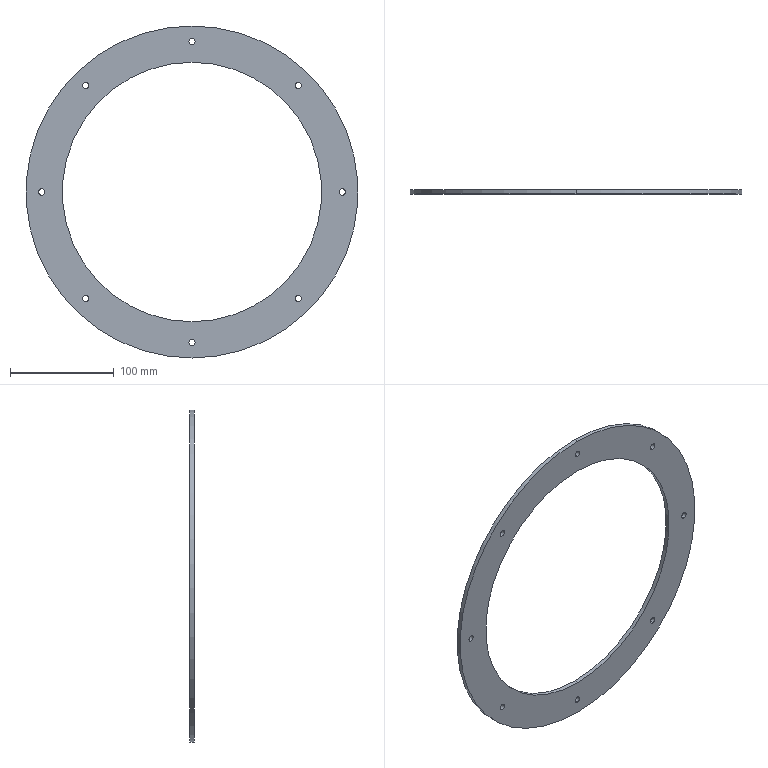Part | SolidWorks | features CirPattern 1, Extrusion 1, ICE 1 | 1 solid | 22 faces | box 320 x 4 x 320 mm | volume 124445 mm3 | cylinder 20 | plane 2 | commonest cylinder face diameters 6 x16 250 x2 320 x2
STEP:
#1=CARTESIAN_POINT('',(-102.53,0.,-105.53));
#2=VERTEX_POINT('',#1);
#3=CARTESIAN_POINT('',(-102.53,0.,-99.53));
#4=VERTEX_POINT('',#3);
#5=CARTESIAN_POINT('',(-102.53,0.,-102.53));
#6=DIRECTION('',(0.,1.,0.));
#7=DIRECTION('',(0.7071,0.,0.7071));
#8=AXIS2_PLACEMENT_3D('',#5,#6,#7);
#9=CIRCLE('',#8,3.);
#10=EDGE_CURVE('',#2,#4,#9,.T.);
#11=ORIENTED_EDGE('',*,*,#10,.F.);
#12=CARTESIAN_POINT('',(-102.53,4.,-105.53));
#13=VERTEX_POINT('',#12);
#14=CARTESIAN_POINT('',(-102.53,0.,-105.53));
#15=DIRECTION('',(0.,1.,0.));
#16=VECTOR('',#15,1000.);
#17=LINE('',#14,#16);
#18=EDGE_CURVE('',#2,#13,#17,.T.);
#19=ORIENTED_EDGE('',*,*,#18,.T.);
#20=CARTESIAN_POINT('',(-102.53,4.,-99.53));
#21=VERTEX_POINT('',#20);
#22=CARTESIAN_POINT('',(-102.53,4.,-102.53));
#23=DIRECTION('',(0.,1.,0.));
#24=DIRECTION('',(0.7071,0.,0.7071));
#25=AXIS2_PLACEMENT_3D('',#22,#23,#24);
#26=CIRCLE('',#25,3.);
#27=EDGE_CURVE('',#13,#21,#26,.T.);
#28=ORIENTED_EDGE('',*,*,#27,.T.);
#29=CARTESIAN_POINT('',(-102.53,0.,-99.53));
#30=DIRECTION('',(0.,1.,0.));
#31=VECTOR('',#30,1000.);
#32=LINE('',#29,#31);
#33=EDGE_CURVE('',#4,#21,#32,.T.);
#34=ORIENTED_EDGE('',*,*,#33,.F.);
#35=EDGE_LOOP('',(#11,#19,#28,#34));
#36=FACE_OUTER_BOUND('',#35,.T.);
#37=CARTESIAN_POINT('',(-102.53,0.,-102.53));
#38=DIRECTION('',(0.,1.,0.));
#39=DIRECTION('',(0.,0.,1.));
#40=AXIS2_PLACEMENT_3D('',#37,#38,#39);
#41=CYLINDRICAL_SURFACE('',#40,3.);
#42=ADVANCED_FACE('',(#36),#41,.F.);
#43=CARTESIAN_POINT('',(-145.,0.,-3.));
#44=VERTEX_POINT('',#43);
#45=CARTESIAN_POINT('',(-145.,0.,3.));
#46=VERTEX_POINT('',#45);
#47=CARTESIAN_POINT('',(-145.,0.,0.));
#48=DIRECTION('',(0.,1.,0.));
#49=DIRECTION('',(1.,0.,0.));
#50=AXIS2_PLACEMENT_3D('',#47,#48,#49);
#51=CIRCLE('',#50,3.);
#52=EDGE_CURVE('',#44,#46,#51,.T.);
#53=ORIENTED_EDGE('',*,*,#52,.F.);
#54=CARTESIAN_POINT('',(-145.,4.,-3.));
#55=VERTEX_POINT('',#54);
#56=CARTESIAN_POINT('',(-145.,0.,-3.));
#57=DIRECTION('',(0.,1.,0.));
#58=VECTOR('',#57,1000.);
#59=LINE('',#56,#58);
#60=EDGE_CURVE('',#44,#55,#59,.T.);
#61=ORIENTED_EDGE('',*,*,#60,.T.);
#62=CARTESIAN_POINT('',(-145.,4.,3.));
#63=VERTEX_POINT('',#62);
#64=CARTESIAN_POINT('',(-145.,4.,0.));
#65=DIRECTION('',(0.,1.,0.));
#66=DIRECTION('',(1.,0.,0.));
#67=AXIS2_PLACEMENT_3D('',#64,#65,#66);
#68=CIRCLE('',#67,3.);
#69=EDGE_CURVE('',#55,#63,#68,.T.);
#70=ORIENTED_EDGE('',*,*,#69,.T.);
#71=CARTESIAN_POINT('',(-145.,0.,3.));
#72=DIRECTION('',(0.,1.,0.));
#73=VECTOR('',#72,1000.);
#74=LINE('',#71,#73);
#75=EDGE_CURVE('',#46,#63,#74,.T.);
#76=ORIENTED_EDGE('',*,*,#75,.F.);
#77=EDGE_LOOP('',(#53,#61,#70,#76));
#78=FACE_OUTER_BOUND('',#77,.T.);
#79=CARTESIAN_POINT('',(-145.,0.,0.));
#80=DIRECTION('',(0.,1.,0.));
#81=DIRECTION('',(0.,0.,1.));
#82=AXIS2_PLACEMENT_3D('',#79,#80,#81);
#83=CYLINDRICAL_SURFACE('',#82,3.);
#84=ADVANCED_FACE('',(#78),#83,.F.);
#85=CARTESIAN_POINT('',(-102.53,0.,99.53));
#86=VERTEX_POINT('',#85);
#87=CARTESIAN_POINT('',(-102.53,0.,105.53));
#88=VERTEX_POINT('',#87);
#89=CARTESIAN_POINT('',(-102.53,0.,102.53));
#90=DIRECTION('',(0.,1.,0.));
#91=DIRECTION('',(0.7071,0.,-0.7071));
#92=AXIS2_PLACEMENT_3D('',#89,#90,#91);
#93=CIRCLE('',#92,3.);
#94=EDGE_CURVE('',#86,#88,#93,.T.);
#95=ORIENTED_EDGE('',*,*,#94,.F.);
#96=CARTESIAN_POINT('',(-102.53,4.,99.53));
#97=VERTEX_POINT('',#96);
#98=CARTESIAN_POINT('',(-102.53,0.,99.53));
#99=DIRECTION('',(0.,1.,0.));
#100=VECTOR('',#99,1000.);
#101=LINE('',#98,#100);
#102=EDGE_CURVE('',#86,#97,#101,.T.);
#103=ORIENTED_EDGE('',*,*,#102,.T.);
#104=CARTESIAN_POINT('',(-102.53,4.,105.53));
#105=VERTEX_POINT('',#104);
#106=CARTESIAN_POINT('',(-102.53,4.,102.53));
#107=DIRECTION('',(0.,1.,0.));
#108=DIRECTION('',(0.7071,0.,-0.7071));
#109=AXIS2_PLACEMENT_3D('',#106,#107,#108);
#110=CIRCLE('',#109,3.);
#111=EDGE_CURVE('',#97,#105,#110,.T.);
#112=ORIENTED_EDGE('',*,*,#111,.T.);
#113=CARTESIAN_POINT('',(-102.53,0.,105.53));
#114=DIRECTION('',(0.,1.,0.));
#115=VECTOR('',#114,1000.);
#116=LINE('',#113,#115);
#117=EDGE_CURVE('',#88,#105,#116,.T.);
#118=ORIENTED_EDGE('',*,*,#117,.F.);
#119=EDGE_LOOP('',(#95,#103,#112,#118));
#120=FACE_OUTER_BOUND('',#119,.T.);
#121=CARTESIAN_POINT('',(-102.53,0.,102.53));
#122=DIRECTION('',(0.,1.,0.));
#123=DIRECTION('',(0.,0.,1.));
#124=AXIS2_PLACEMENT_3D('',#121,#122,#123);
#125=CYLINDRICAL_SURFACE('',#124,3.);
#126=ADVANCED_FACE('',(#120),#125,.F.);
#127=CARTESIAN_POINT('',(0.,0.,142.));
#128=VERTEX_POINT('',#127);
#129=CARTESIAN_POINT('',(0.,0.,148.));
#130=VERTEX_POINT('',#129);
#131=CARTESIAN_POINT('',(0.,0.,145.));
#132=DIRECTION('',(0.,1.,0.));
#133=DIRECTION('',(0.,0.,-1.));
#134=AXIS2_PLACEMENT_3D('',#131,#132,#133);
#135=CIRCLE('',#134,3.);
#136=EDGE_CURVE('',#128,#130,#135,.T.);
#137=ORIENTED_EDGE('',*,*,#136,.F.);
#138=CARTESIAN_POINT('',(0.,4.,142.));
#139=VERTEX_POINT('',#138);
#140=CARTESIAN_POINT('',(0.,0.,142.));
#141=DIRECTION('',(0.,1.,0.));
#142=VECTOR('',#141,1000.);
#143=LINE('',#140,#142);
#144=EDGE_CURVE('',#128,#139,#143,.T.);
#145=ORIENTED_EDGE('',*,*,#144,.T.);
#146=CARTESIAN_POINT('',(0.,4.,148.));
#147=VERTEX_POINT('',#146);
#148=CARTESIAN_POINT('',(0.,4.,145.));
#149=DIRECTION('',(0.,1.,0.));
#150=DIRECTION('',(0.,0.,-1.));
#151=AXIS2_PLACEMENT_3D('',#148,#149,#150);
#152=CIRCLE('',#151,3.);
#153=EDGE_CURVE('',#139,#147,#152,.T.);
#154=ORIENTED_EDGE('',*,*,#153,.T.);
#155=CARTESIAN_POINT('',(0.,0.,148.));
#156=DIRECTION('',(0.,1.,0.));
#157=VECTOR('',#156,1000.);
#158=LINE('',#155,#157);
#159=EDGE_CURVE('',#130,#147,#158,.T.);
#160=ORIENTED_EDGE('',*,*,#159,.F.);
#161=EDGE_LOOP('',(#137,#145,#154,#160));
#162=FACE_OUTER_BOUND('',#161,.T.);
#163=CARTESIAN_POINT('',(0.,0.,145.));
#164=DIRECTION('',(0.,1.,0.));
#165=DIRECTION('',(0.,0.,1.));
#166=AXIS2_PLACEMENT_3D('',#163,#164,#165);
#167=CYLINDRICAL_SURFACE('',#166,3.);
#168=ADVANCED_FACE('',(#162),#167,.F.);
#169=CARTESIAN_POINT('',(102.53,0.,99.53));
#170=VERTEX_POINT('',#169);
#171=CARTESIAN_POINT('',(102.53,0.,105.53));
#172=VERTEX_POINT('',#171);
#173=CARTESIAN_POINT('',(102.53,0.,102.53));
#174=DIRECTION('',(0.,1.,0.));
#175=DIRECTION('',(-0.7071,0.,-0.7071));
#176=AXIS2_PLACEMENT_3D('',#173,#174,#175);
#177=CIRCLE('',#176,3.);
#178=EDGE_CURVE('',#170,#172,#177,.T.);
#179=ORIENTED_EDGE('',*,*,#178,.F.);
#180=CARTESIAN_POINT('',(102.53,4.,99.53));
#181=VERTEX_POINT('',#180);
#182=CARTESIAN_POINT('',(102.53,0.,99.53));
#183=DIRECTION('',(0.,1.,0.));
#184=VECTOR('',#183,1000.);
#185=LINE('',#182,#184);
#186=EDGE_CURVE('',#170,#181,#185,.T.);
#187=ORIENTED_EDGE('',*,*,#186,.T.);
#188=CARTESIAN_POINT('',(102.53,4.,105.53));
#189=VERTEX_POINT('',#188);
#190=CARTESIAN_POINT('',(102.53,4.,102.53));
#191=DIRECTION('',(0.,1.,0.));
#192=DIRECTION('',(-0.7071,0.,-0.7071));
#193=AXIS2_PLACEMENT_3D('',#190,#191,#192);
#194=CIRCLE('',#193,3.);
#195=EDGE_CURVE('',#181,#189,#194,.T.);
#196=ORIENTED_EDGE('',*,*,#195,.T.);
#197=CARTESIAN_POINT('',(102.53,0.,105.53));
#198=DIRECTION('',(0.,1.,0.));
#199=VECTOR('',#198,1000.);
#200=LINE('',#197,#199);
#201=EDGE_CURVE('',#172,#189,#200,.T.);
#202=ORIENTED_EDGE('',*,*,#201,.F.);
#203=EDGE_LOOP('',(#179,#187,#196,#202));
#204=FACE_OUTER_BOUND('',#203,.T.);
#205=CARTESIAN_POINT('',(102.53,0.,102.53));
#206=DIRECTION('',(0.,1.,0.));
#207=DIRECTION('',(0.,0.,1.));
#208=AXIS2_PLACEMENT_3D('',#205,#206,#207);
#209=CYLINDRICAL_SURFACE('',#208,3.);
#210=ADVANCED_FACE('',(#204),#209,.F.);
#211=CARTESIAN_POINT('',(145.,0.,-3.));
#212=VERTEX_POINT('',#211);
#213=CARTESIAN_POINT('',(145.,0.,3.));
#214=VERTEX_POINT('',#213);
#215=CARTESIAN_POINT('',(145.,0.,0.));
#216=DIRECTION('',(0.,1.,0.));
#217=DIRECTION('',(-1.,0.,0.));
#218=AXIS2_PLACEMENT_3D('',#215,#216,#217);
#219=CIRCLE('',#218,3.);
#220=EDGE_CURVE('',#212,#214,#219,.T.);
#221=ORIENTED_EDGE('',*,*,#220,.F.);
#222=CARTESIAN_POINT('',(145.,4.,-3.));
#223=VERTEX_POINT('',#222);
#224=CARTESIAN_POINT('',(145.,0.,-3.));
#225=DIRECTION('',(0.,1.,0.));
#226=VECTOR('',#225,1000.);
#227=LINE('',#224,#226);
#228=EDGE_CURVE('',#212,#223,#227,.T.);
#229=ORIENTED_EDGE('',*,*,#228,.T.);
#230=CARTESIAN_POINT('',(145.,4.,3.));
#231=VERTEX_POINT('',#230);
#232=CARTESIAN_POINT('',(145.,4.,0.));
#233=DIRECTION('',(0.,1.,0.));
#234=DIRECTION('',(-1.,0.,0.));
#235=AXIS2_PLACEMENT_3D('',#232,#233,#234);
#236=CIRCLE('',#235,3.);
#237=EDGE_CURVE('',#223,#231,#236,.T.);
#238=ORIENTED_EDGE('',*,*,#237,.T.);
#239=CARTESIAN_POINT('',(145.,0.,3.));
#240=DIRECTION('',(0.,1.,0.));
#241=VECTOR('',#240,1000.);
#242=LINE('',#239,#241);
#243=EDGE_CURVE('',#214,#231,#242,.T.);
#244=ORIENTED_EDGE('',*,*,#243,.F.);
#245=EDGE_LOOP('',(#221,#229,#238,#244));
#246=FACE_OUTER_BOUND('',#245,.T.);
#247=CARTESIAN_POINT('',(145.,0.,0.));
#248=DIRECTION('',(0.,1.,0.));
#249=DIRECTION('',(0.,0.,1.));
#250=AXIS2_PLACEMENT_3D('',#247,#248,#249);
#251=CYLINDRICAL_SURFACE('',#250,3.);
#252=ADVANCED_FACE('',(#246),#251,.F.);
#253=CARTESIAN_POINT('',(102.53,0.,-105.53));
#254=VERTEX_POINT('',#253);
#255=CARTESIAN_POINT('',(102.53,0.,-99.53));
#256=VERTEX_POINT('',#255);
#257=CARTESIAN_POINT('',(102.53,0.,-102.53));
#258=DIRECTION('',(0.,1.,0.));
#259=DIRECTION('',(-0.7071,0.,0.7071));
#260=AXIS2_PLACEMENT_3D('',#257,#258,#259);
#261=CIRCLE('',#260,3.);
#262=EDGE_CURVE('',#254,#256,#261,.T.);
#263=ORIENTED_EDGE('',*,*,#262,.F.);
#264=CARTESIAN_POINT('',(102.53,4.,-105.53));
#265=VERTEX_POINT('',#264);
#266=CARTESIAN_POINT('',(102.53,0.,-105.53));
#267=DIRECTION('',(0.,1.,0.));
#268=VECTOR('',#267,1000.);
#269=LINE('',#266,#268);
#270=EDGE_CURVE('',#254,#265,#269,.T.);
#271=ORIENTED_EDGE('',*,*,#270,.T.);
#272=CARTESIAN_POINT('',(102.53,4.,-99.53));
#273=VERTEX_POINT('',#272);
#274=CARTESIAN_POINT('',(102.53,4.,-102.53));
#275=DIRECTION('',(0.,1.,0.));
#276=DIRECTION('',(-0.7071,0.,0.7071));
#277=AXIS2_PLACEMENT_3D('',#274,#275,#276);
#278=CIRCLE('',#277,3.);
#279=EDGE_CURVE('',#265,#273,#278,.T.);
#280=ORIENTED_EDGE('',*,*,#279,.T.);
#281=CARTESIAN_POINT('',(102.53,0.,-99.53));
#282=DIRECTION('',(0.,1.,0.));
#283=VECTOR('',#282,1000.);
#284=LINE('',#281,#283);
#285=EDGE_CURVE('',#256,#273,#284,.T.);
#286=ORIENTED_EDGE('',*,*,#285,.F.);
#287=EDGE_LOOP('',(#263,#271,#280,#286));
#288=FACE_OUTER_BOUND('',#287,.T.);
#289=CARTESIAN_POINT('',(102.53,0.,-102.53));
#290=DIRECTION('',(0.,1.,0.));
#291=DIRECTION('',(0.,0.,1.));
#292=AXIS2_PLACEMENT_3D('',#289,#290,#291);
#293=CYLINDRICAL_SURFACE('',#292,3.);
#294=ADVANCED_FACE('',(#288),#293,.F.);
#295=CARTESIAN_POINT('',(0.,0.,-148.));
#296=VERTEX_POINT('',#295);
#297=CARTESIAN_POINT('',(0.,0.,-142.));
#298=VERTEX_POINT('',#297);
#299=CARTESIAN_POINT('',(0.,0.,-145.));
#300=DIRECTION('',(0.,1.,0.));
#301=DIRECTION('',(0.,0.,1.));
#302=AXIS2_PLACEMENT_3D('',#299,#300,#301);
#303=CIRCLE('',#302,3.);
#304=EDGE_CURVE('',#296,#298,#303,.T.);
#305=ORIENTED_EDGE('',*,*,#304,.F.);
#306=CARTESIAN_POINT('',(0.,4.,-148.));
#307=VERTEX_POINT('',#306);
#308=CARTESIAN_POINT('',(0.,0.,-148.));
#309=DIRECTION('',(0.,1.,0.));
#310=VECTOR('',#309,1000.);
#311=LINE('',#308,#310);
#312=EDGE_CURVE('',#296,#307,#311,.T.);
#313=ORIENTED_EDGE('',*,*,#312,.T.);
#314=CARTESIAN_POINT('',(0.,4.,-142.));
#315=VERTEX_POINT('',#314);
#316=CARTESIAN_POINT('',(0.,4.,-145.));
#317=DIRECTION('',(0.,1.,0.));
#318=DIRECTION('',(0.,0.,1.));
#319=AXIS2_PLACEMENT_3D('',#316,#317,#318);
#320=CIRCLE('',#319,3.);
#321=EDGE_CURVE('',#307,#315,#320,.T.);
#322=ORIENTED_EDGE('',*,*,#321,.T.);
#323=CARTESIAN_POINT('',(0.,0.,-142.));
#324=DIRECTION('',(0.,1.,0.));
#325=VECTOR('',#324,1000.);
#326=LINE('',#323,#325);
#327=EDGE_CURVE('',#298,#315,#326,.T.);
#328=ORIENTED_EDGE('',*,*,#327,.F.);
#329=EDGE_LOOP('',(#305,#313,#322,#328));
#330=FACE_OUTER_BOUND('',#329,.T.);
#331=CARTESIAN_POINT('',(0.,0.,-145.));
#332=DIRECTION('',(0.,1.,0.));
#333=DIRECTION('',(0.,0.,1.));
#334=AXIS2_PLACEMENT_3D('',#331,#332,#333);
#335=CYLINDRICAL_SURFACE('',#334,3.);
#336=ADVANCED_FACE('',(#330),#335,.F.);
#337=CARTESIAN_POINT('',(0.,4.,-125.));
#338=VERTEX_POINT('',#337);
#339=CARTESIAN_POINT('',(0.,4.,125.));
#340=VERTEX_POINT('',#339);
#341=CARTESIAN_POINT('',(0.,4.,0.));
#342=DIRECTION('',(0.,1.,0.));
#343=DIRECTION('',(0.,0.,1.));
#344=AXIS2_PLACEMENT_3D('',#341,#342,#343);
#345=CIRCLE('',#344,125.);
#346=EDGE_CURVE('',#338,#340,#345,.T.);
#347=ORIENTED_EDGE('',*,*,#346,.T.);
#348=CARTESIAN_POINT('',(0.,0.,125.));
#349=VERTEX_POINT('',#348);
#350=CARTESIAN_POINT('',(0.,4.,125.));
#351=DIRECTION('',(0.,-1.,0.));
#352=VECTOR('',#351,1000.);
#353=LINE('',#350,#352);
#354=EDGE_CURVE('',#340,#349,#353,.T.);
#355=ORIENTED_EDGE('',*,*,#354,.T.);
#356=CARTESIAN_POINT('',(0.,0.,-125.));
#357=VERTEX_POINT('',#356);
#358=CARTESIAN_POINT('',(0.,0.,0.));
#359=DIRECTION('',(0.,1.,0.));
#360=DIRECTION('',(0.,0.,1.));
#361=AXIS2_PLACEMENT_3D('',#358,#359,#360);
#362=CIRCLE('',#361,125.);
#363=EDGE_CURVE('',#357,#349,#362,.T.);
#364=ORIENTED_EDGE('',*,*,#363,.F.);
#365=CARTESIAN_POINT('',(0.,4.,-125.));
#366=DIRECTION('',(0.,-1.,0.));
#367=VECTOR('',#366,1000.);
#368=LINE('',#365,#367);
#369=EDGE_CURVE('',#338,#357,#368,.T.);
#370=ORIENTED_EDGE('',*,*,#369,.F.);
#371=EDGE_LOOP('',(#347,#355,#364,#370));
#372=FACE_OUTER_BOUND('',#371,.T.);
#373=CARTESIAN_POINT('',(0.,4.,0.));
#374=DIRECTION('',(0.,-1.,0.));
#375=DIRECTION('',(0.,0.,-1.));
#376=AXIS2_PLACEMENT_3D('',#373,#374,#375);
#377=CYLINDRICAL_SURFACE('',#376,125.);
#378=ADVANCED_FACE('',(#372),#377,.F.);
#379=CARTESIAN_POINT('',(0.,4.,160.));
#380=VERTEX_POINT('',#379);
#381=CARTESIAN_POINT('',(0.,4.,-160.));
#382=VERTEX_POINT('',#381);
#383=CARTESIAN_POINT('',(0.,4.,0.));
#384=DIRECTION('',(0.,1.,0.));
#385=DIRECTION('',(0.,0.,1.));
#386=AXIS2_PLACEMENT_3D('',#383,#384,#385);
#387=CIRCLE('',#386,160.);
#388=EDGE_CURVE('',#380,#382,#387,.T.);
#389=ORIENTED_EDGE('',*,*,#388,.F.);
#390=CARTESIAN_POINT('',(0.,0.,160.));
#391=VERTEX_POINT('',#390);
#392=CARTESIAN_POINT('',(0.,4.,160.));
#393=DIRECTION('',(0.,-1.,0.));
#394=VECTOR('',#393,1000.);
#395=LINE('',#392,#394);
#396=EDGE_CURVE('',#380,#391,#395,.T.);
#397=ORIENTED_EDGE('',*,*,#396,.T.);
#398=CARTESIAN_POINT('',(0.,0.,-160.));
#399=VERTEX_POINT('',#398);
#400=CARTESIAN_POINT('',(0.,0.,0.));
#401=DIRECTION('',(0.,1.,0.));
#402=DIRECTION('',(0.,0.,1.));
#403=AXIS2_PLACEMENT_3D('',#400,#401,#402);
#404=CIRCLE('',#403,160.);
#405=EDGE_CURVE('',#391,#399,#404,.T.);
#406=ORIENTED_EDGE('',*,*,#405,.T.);
#407=CARTESIAN_POINT('',(0.,4.,-160.));
#408=DIRECTION('',(0.,-1.,0.));
#409=VECTOR('',#408,1000.);
#410=LINE('',#407,#409);
#411=EDGE_CURVE('',#382,#399,#410,.T.);
#412=ORIENTED_EDGE('',*,*,#411,.F.);
#413=EDGE_LOOP('',(#389,#397,#406,#412));
#414=FACE_OUTER_BOUND('',#413,.T.);
#415=CARTESIAN_POINT('',(0.,4.,0.));
#416=DIRECTION('',(0.,-1.,0.));
#417=DIRECTION('',(0.,0.,-1.));
#418=AXIS2_PLACEMENT_3D('',#415,#416,#417);
#419=CYLINDRICAL_SURFACE('',#418,160.);
#420=ADVANCED_FACE('',(#414),#419,.T.);
#421=CARTESIAN_POINT('',(-102.53,4.,-102.53));
#422=DIRECTION('',(0.,1.,0.));
#423=DIRECTION('',(0.7071,0.,0.7071));
#424=AXIS2_PLACEMENT_3D('',#421,#422,#423);
#425=CIRCLE('',#424,3.);
#426=EDGE_CURVE('',#21,#13,#425,.T.);
#427=ORIENTED_EDGE('',*,*,#426,.F.);
#428=ORIENTED_EDGE('',*,*,#27,.F.);
#429=EDGE_LOOP('',(#427,#428));
#430=FACE_BOUND('',#429,.T.);
#431=CARTESIAN_POINT('',(-145.,4.,0.));
#432=DIRECTION('',(0.,1.,0.));
#433=DIRECTION('',(1.,0.,0.));
#434=AXIS2_PLACEMENT_3D('',#431,#432,#433);
#435=CIRCLE('',#434,3.);
#436=EDGE_CURVE('',#63,#55,#435,.T.);
#437=ORIENTED_EDGE('',*,*,#436,.F.);
#438=ORIENTED_EDGE('',*,*,#69,.F.);
#439=EDGE_LOOP('',(#437,#438));
#440=FACE_BOUND('',#439,.T.);
#441=CARTESIAN_POINT('',(-102.53,4.,102.53));
#442=DIRECTION('',(0.,1.,0.));
#443=DIRECTION('',(0.7071,0.,-0.7071));
#444=AXIS2_PLACEMENT_3D('',#441,#442,#443);
#445=CIRCLE('',#444,3.);
#446=EDGE_CURVE('',#105,#97,#445,.T.);
#447=ORIENTED_EDGE('',*,*,#446,.F.);
#448=ORIENTED_EDGE('',*,*,#111,.F.);
#449=EDGE_LOOP('',(#447,#448));
#450=FACE_BOUND('',#449,.T.);
#451=CARTESIAN_POINT('',(0.,4.,145.));
#452=DIRECTION('',(0.,1.,0.));
#453=DIRECTION('',(0.,0.,-1.));
#454=AXIS2_PLACEMENT_3D('',#451,#452,#453);
#455=CIRCLE('',#454,3.);
#456=EDGE_CURVE('',#147,#139,#455,.T.);
#457=ORIENTED_EDGE('',*,*,#456,.F.);
#458=ORIENTED_EDGE('',*,*,#153,.F.);
#459=EDGE_LOOP('',(#457,#458));
#460=FACE_BOUND('',#459,.T.);
#461=CARTESIAN_POINT('',(102.53,4.,102.53));
#462=DIRECTION('',(0.,1.,0.));
#463=DIRECTION('',(-0.7071,0.,-0.7071));
#464=AXIS2_PLACEMENT_3D('',#461,#462,#463);
#465=CIRCLE('',#464,3.);
#466=EDGE_CURVE('',#189,#181,#465,.T.);
#467=ORIENTED_EDGE('',*,*,#466,.F.);
#468=ORIENTED_EDGE('',*,*,#195,.F.);
#469=EDGE_LOOP('',(#467,#468));
#470=FACE_BOUND('',#469,.T.);
#471=CARTESIAN_POINT('',(145.,4.,0.));
#472=DIRECTION('',(0.,1.,0.));
#473=DIRECTION('',(-1.,0.,0.));
#474=AXIS2_PLACEMENT_3D('',#471,#472,#473);
#475=CIRCLE('',#474,3.);
#476=EDGE_CURVE('',#231,#223,#475,.T.);
#477=ORIENTED_EDGE('',*,*,#476,.F.);
#478=ORIENTED_EDGE('',*,*,#237,.F.);
#479=EDGE_LOOP('',(#477,#478));
#480=FACE_BOUND('',#479,.T.);
#481=CARTESIAN_POINT('',(102.53,4.,-102.53));
#482=DIRECTION('',(0.,1.,0.));
#483=DIRECTION('',(-0.7071,0.,0.7071));
#484=AXIS2_PLACEMENT_3D('',#481,#482,#483);
#485=CIRCLE('',#484,3.);
#486=EDGE_CURVE('',#273,#265,#485,.T.);
#487=ORIENTED_EDGE('',*,*,#486,.F.);
#488=ORIENTED_EDGE('',*,*,#279,.F.);
#489=EDGE_LOOP('',(#487,#488));
#490=FACE_BOUND('',#489,.T.);
#491=CARTESIAN_POINT('',(0.,4.,-145.));
#492=DIRECTION('',(0.,1.,0.));
#493=DIRECTION('',(0.,0.,1.));
#494=AXIS2_PLACEMENT_3D('',#491,#492,#493);
#495=CIRCLE('',#494,3.);
#496=EDGE_CURVE('',#315,#307,#495,.T.);
#497=ORIENTED_EDGE('',*,*,#496,.F.);
#498=ORIENTED_EDGE('',*,*,#321,.F.);
#499=EDGE_LOOP('',(#497,#498));
#500=FACE_BOUND('',#499,.T.);
#501=CARTESIAN_POINT('',(0.,4.,0.));
#502=DIRECTION('',(0.,1.,0.));
#503=DIRECTION('',(0.,0.,1.));
#504=AXIS2_PLACEMENT_3D('',#501,#502,#503);
#505=CIRCLE('',#504,160.);
#506=EDGE_CURVE('',#382,#380,#505,.T.);
#507=ORIENTED_EDGE('',*,*,#506,.T.);
#508=ORIENTED_EDGE('',*,*,#388,.T.);
#509=EDGE_LOOP('',(#507,#508));
#510=FACE_OUTER_BOUND('',#509,.T.);
#511=ORIENTED_EDGE('',*,*,#346,.F.);
#512=CARTESIAN_POINT('',(0.,4.,0.));
#513=DIRECTION('',(0.,1.,0.));
#514=DIRECTION('',(0.,0.,1.));
#515=AXIS2_PLACEMENT_3D('',#512,#513,#514);
#516=CIRCLE('',#515,125.);
#517=EDGE_CURVE('',#340,#338,#516,.T.);
#518=ORIENTED_EDGE('',*,*,#517,.F.);
#519=EDGE_LOOP('',(#511,#518));
#520=FACE_BOUND('',#519,.T.);
#521=CARTESIAN_POINT('',(0.,4.,0.));
#522=DIRECTION('',(0.,1.,0.));
#523=DIRECTION('',(0.,0.,1.));
#524=AXIS2_PLACEMENT_3D('',#521,#522,#523);
#525=PLANE('',#524);
#526=ADVANCED_FACE('',(#430,#440,#450,#460,#470,#480,#490,#500,#510,#520),#525,.T.);
#527=CARTESIAN_POINT('',(-102.53,0.,-102.53));
#528=DIRECTION('',(0.,1.,0.));
#529=DIRECTION('',(0.7071,0.,0.7071));
#530=AXIS2_PLACEMENT_3D('',#527,#528,#529);
#531=CIRCLE('',#530,3.);
#532=EDGE_CURVE('',#4,#2,#531,.T.);
#533=ORIENTED_EDGE('',*,*,#532,.T.);
#534=ORIENTED_EDGE('',*,*,#10,.T.);
#535=EDGE_LOOP('',(#533,#534));
#536=FACE_BOUND('',#535,.T.);
#537=CARTESIAN_POINT('',(-145.,0.,0.));
#538=DIRECTION('',(0.,1.,0.));
#539=DIRECTION('',(1.,0.,0.));
#540=AXIS2_PLACEMENT_3D('',#537,#538,#539);
#541=CIRCLE('',#540,3.);
#542=EDGE_CURVE('',#46,#44,#541,.T.);
#543=ORIENTED_EDGE('',*,*,#542,.T.);
#544=ORIENTED_EDGE('',*,*,#52,.T.);
#545=EDGE_LOOP('',(#543,#544));
#546=FACE_BOUND('',#545,.T.);
#547=CARTESIAN_POINT('',(-102.53,0.,102.53));
#548=DIRECTION('',(0.,1.,0.));
#549=DIRECTION('',(0.7071,0.,-0.7071));
#550=AXIS2_PLACEMENT_3D('',#547,#548,#549);
#551=CIRCLE('',#550,3.);
#552=EDGE_CURVE('',#88,#86,#551,.T.);
#553=ORIENTED_EDGE('',*,*,#552,.T.);
#554=ORIENTED_EDGE('',*,*,#94,.T.);
#555=EDGE_LOOP('',(#553,#554));
#556=FACE_BOUND('',#555,.T.);
#557=CARTESIAN_POINT('',(0.,0.,145.));
#558=DIRECTION('',(0.,1.,0.));
#559=DIRECTION('',(0.,0.,-1.));
#560=AXIS2_PLACEMENT_3D('',#557,#558,#559);
#561=CIRCLE('',#560,3.);
#562=EDGE_CURVE('',#130,#128,#561,.T.);
#563=ORIENTED_EDGE('',*,*,#562,.T.);
#564=ORIENTED_EDGE('',*,*,#136,.T.);
#565=EDGE_LOOP('',(#563,#564));
#566=FACE_BOUND('',#565,.T.);
#567=CARTESIAN_POINT('',(102.53,0.,102.53));
#568=DIRECTION('',(0.,1.,0.));
#569=DIRECTION('',(-0.7071,0.,-0.7071));
#570=AXIS2_PLACEMENT_3D('',#567,#568,#569);
#571=CIRCLE('',#570,3.);
#572=EDGE_CURVE('',#172,#170,#571,.T.);
#573=ORIENTED_EDGE('',*,*,#572,.T.);
#574=ORIENTED_EDGE('',*,*,#178,.T.);
#575=EDGE_LOOP('',(#573,#574));
#576=FACE_BOUND('',#575,.T.);
#577=CARTESIAN_POINT('',(145.,0.,0.));
#578=DIRECTION('',(0.,1.,0.));
#579=DIRECTION('',(-1.,0.,0.));
#580=AXIS2_PLACEMENT_3D('',#577,#578,#579);
#581=CIRCLE('',#580,3.);
#582=EDGE_CURVE('',#214,#212,#581,.T.);
#583=ORIENTED_EDGE('',*,*,#582,.T.);
#584=ORIENTED_EDGE('',*,*,#220,.T.);
#585=EDGE_LOOP('',(#583,#584));
#586=FACE_BOUND('',#585,.T.);
#587=CARTESIAN_POINT('',(102.53,0.,-102.53));
#588=DIRECTION('',(0.,1.,0.));
#589=DIRECTION('',(-0.7071,0.,0.7071));
#590=AXIS2_PLACEMENT_3D('',#587,#588,#589);
#591=CIRCLE('',#590,3.);
#592=EDGE_CURVE('',#256,#254,#591,.T.);
#593=ORIENTED_EDGE('',*,*,#592,.T.);
#594=ORIENTED_EDGE('',*,*,#262,.T.);
#595=EDGE_LOOP('',(#593,#594));
#596=FACE_BOUND('',#595,.T.);
#597=CARTESIAN_POINT('',(0.,0.,-145.));
#598=DIRECTION('',(0.,1.,0.));
#599=DIRECTION('',(0.,0.,1.));
#600=AXIS2_PLACEMENT_3D('',#597,#598,#599);
#601=CIRCLE('',#600,3.);
#602=EDGE_CURVE('',#298,#296,#601,.T.);
#603=ORIENTED_EDGE('',*,*,#602,.T.);
#604=ORIENTED_EDGE('',*,*,#304,.T.);
#605=EDGE_LOOP('',(#603,#604));
#606=FACE_BOUND('',#605,.T.);
#607=CARTESIAN_POINT('',(0.,0.,0.));
#608=DIRECTION('',(0.,1.,0.));
#609=DIRECTION('',(0.,0.,1.));
#610=AXIS2_PLACEMENT_3D('',#607,#608,#609);
#611=CIRCLE('',#610,160.);
#612=EDGE_CURVE('',#399,#391,#611,.T.);
#613=ORIENTED_EDGE('',*,*,#612,.F.);
#614=ORIENTED_EDGE('',*,*,#405,.F.);
#615=EDGE_LOOP('',(#613,#614));
#616=FACE_OUTER_BOUND('',#615,.T.);
#617=ORIENTED_EDGE('',*,*,#363,.T.);
#618=CARTESIAN_POINT('',(0.,0.,0.));
#619=DIRECTION('',(0.,1.,0.));
#620=DIRECTION('',(0.,0.,1.));
#621=AXIS2_PLACEMENT_3D('',#618,#619,#620);
#622=CIRCLE('',#621,125.);
#623=EDGE_CURVE('',#349,#357,#622,.T.);
#624=ORIENTED_EDGE('',*,*,#623,.T.);
#625=EDGE_LOOP('',(#617,#624));
#626=FACE_BOUND('',#625,.T.);
#627=CARTESIAN_POINT('',(0.,0.,0.));
#628=DIRECTION('',(0.,1.,0.));
#629=DIRECTION('',(0.,0.,1.));
#630=AXIS2_PLACEMENT_3D('',#627,#628,#629);
#631=PLANE('',#630);
#632=ADVANCED_FACE('',(#536,#546,#556,#566,#576,#586,#596,#606,#616,#626),#631,.F.);
#633=ORIENTED_EDGE('',*,*,#396,.F.);
#634=ORIENTED_EDGE('',*,*,#506,.F.);
#635=ORIENTED_EDGE('',*,*,#411,.T.);
#636=ORIENTED_EDGE('',*,*,#612,.T.);
#637=EDGE_LOOP('',(#633,#634,#635,#636));
#638=FACE_OUTER_BOUND('',#637,.T.);
#639=CARTESIAN_POINT('',(0.,4.,0.));
#640=DIRECTION('',(0.,-1.,0.));
#641=DIRECTION('',(0.,0.,-1.));
#642=AXIS2_PLACEMENT_3D('',#639,#640,#641);
#643=CYLINDRICAL_SURFACE('',#642,160.);
#644=ADVANCED_FACE('',(#638),#643,.T.);
#645=ORIENTED_EDGE('',*,*,#354,.F.);
#646=ORIENTED_EDGE('',*,*,#517,.T.);
#647=ORIENTED_EDGE('',*,*,#369,.T.);
#648=ORIENTED_EDGE('',*,*,#623,.F.);
#649=EDGE_LOOP('',(#645,#646,#647,#648));
#650=FACE_OUTER_BOUND('',#649,.T.);
#651=CARTESIAN_POINT('',(0.,4.,0.));
#652=DIRECTION('',(0.,-1.,0.));
#653=DIRECTION('',(0.,0.,-1.));
#654=AXIS2_PLACEMENT_3D('',#651,#652,#653);
#655=CYLINDRICAL_SURFACE('',#654,125.);
#656=ADVANCED_FACE('',(#650),#655,.F.);
#657=ORIENTED_EDGE('',*,*,#312,.F.);
#658=ORIENTED_EDGE('',*,*,#602,.F.);
#659=ORIENTED_EDGE('',*,*,#327,.T.);
#660=ORIENTED_EDGE('',*,*,#496,.T.);
#661=EDGE_LOOP('',(#657,#658,#659,#660));
#662=FACE_OUTER_BOUND('',#661,.T.);
#663=CARTESIAN_POINT('',(0.,0.,-145.));
#664=DIRECTION('',(0.,1.,0.));
#665=DIRECTION('',(0.,0.,1.));
#666=AXIS2_PLACEMENT_3D('',#663,#664,#665);
#667=CYLINDRICAL_SURFACE('',#666,3.);
#668=ADVANCED_FACE('',(#662),#667,.F.);
#669=ORIENTED_EDGE('',*,*,#270,.F.);
#670=ORIENTED_EDGE('',*,*,#592,.F.);
#671=ORIENTED_EDGE('',*,*,#285,.T.);
#672=ORIENTED_EDGE('',*,*,#486,.T.);
#673=EDGE_LOOP('',(#669,#670,#671,#672));
#674=FACE_OUTER_BOUND('',#673,.T.);
#675=CARTESIAN_POINT('',(102.53,0.,-102.53));
#676=DIRECTION('',(0.,1.,0.));
#677=DIRECTION('',(0.,0.,1.));
#678=AXIS2_PLACEMENT_3D('',#675,#676,#677);
#679=CYLINDRICAL_SURFACE('',#678,3.);
#680=ADVANCED_FACE('',(#674),#679,.F.);
#681=ORIENTED_EDGE('',*,*,#228,.F.);
#682=ORIENTED_EDGE('',*,*,#582,.F.);
#683=ORIENTED_EDGE('',*,*,#243,.T.);
#684=ORIENTED_EDGE('',*,*,#476,.T.);
#685=EDGE_LOOP('',(#681,#682,#683,#684));
#686=FACE_OUTER_BOUND('',#685,.T.);
#687=CARTESIAN_POINT('',(145.,0.,0.));
#688=DIRECTION('',(0.,1.,0.));
#689=DIRECTION('',(0.,0.,1.));
#690=AXIS2_PLACEMENT_3D('',#687,#688,#689);
#691=CYLINDRICAL_SURFACE('',#690,3.);
#692=ADVANCED_FACE('',(#686),#691,.F.);
#693=ORIENTED_EDGE('',*,*,#186,.F.);
#694=ORIENTED_EDGE('',*,*,#572,.F.);
#695=ORIENTED_EDGE('',*,*,#201,.T.);
#696=ORIENTED_EDGE('',*,*,#466,.T.);
#697=EDGE_LOOP('',(#693,#694,#695,#696));
#698=FACE_OUTER_BOUND('',#697,.T.);
#699=CARTESIAN_POINT('',(102.53,0.,102.53));
#700=DIRECTION('',(0.,1.,0.));
#701=DIRECTION('',(0.,0.,1.));
#702=AXIS2_PLACEMENT_3D('',#699,#700,#701);
#703=CYLINDRICAL_SURFACE('',#702,3.);
#704=ADVANCED_FACE('',(#698),#703,.F.);
#705=ORIENTED_EDGE('',*,*,#144,.F.);
#706=ORIENTED_EDGE('',*,*,#562,.F.);
#707=ORIENTED_EDGE('',*,*,#159,.T.);
#708=ORIENTED_EDGE('',*,*,#456,.T.);
#709=EDGE_LOOP('',(#705,#706,#707,#708));
#710=FACE_OUTER_BOUND('',#709,.T.);
#711=CARTESIAN_POINT('',(0.,0.,145.));
#712=DIRECTION('',(0.,1.,0.));
#713=DIRECTION('',(0.,0.,1.));
#714=AXIS2_PLACEMENT_3D('',#711,#712,#713);
#715=CYLINDRICAL_SURFACE('',#714,3.);
#716=ADVANCED_FACE('',(#710),#715,.F.);
#717=ORIENTED_EDGE('',*,*,#102,.F.);
#718=ORIENTED_EDGE('',*,*,#552,.F.);
#719=ORIENTED_EDGE('',*,*,#117,.T.);
#720=ORIENTED_EDGE('',*,*,#446,.T.);
#721=EDGE_LOOP('',(#717,#718,#719,#720));
#722=FACE_OUTER_BOUND('',#721,.T.);
#723=CARTESIAN_POINT('',(-102.53,0.,102.53));
#724=DIRECTION('',(0.,1.,0.));
#725=DIRECTION('',(0.,0.,1.));
#726=AXIS2_PLACEMENT_3D('',#723,#724,#725);
#727=CYLINDRICAL_SURFACE('',#726,3.);
#728=ADVANCED_FACE('',(#722),#727,.F.);
#729=ORIENTED_EDGE('',*,*,#60,.F.);
#730=ORIENTED_EDGE('',*,*,#542,.F.);
#731=ORIENTED_EDGE('',*,*,#75,.T.);
#732=ORIENTED_EDGE('',*,*,#436,.T.);
#733=EDGE_LOOP('',(#729,#730,#731,#732));
#734=FACE_OUTER_BOUND('',#733,.T.);
#735=CARTESIAN_POINT('',(-145.,0.,0.));
#736=DIRECTION('',(0.,1.,0.));
#737=DIRECTION('',(0.,0.,1.));
#738=AXIS2_PLACEMENT_3D('',#735,#736,#737);
#739=CYLINDRICAL_SURFACE('',#738,3.);
#740=ADVANCED_FACE('',(#734),#739,.F.);
#741=ORIENTED_EDGE('',*,*,#18,.F.);
#742=ORIENTED_EDGE('',*,*,#532,.F.);
#743=ORIENTED_EDGE('',*,*,#33,.T.);
#744=ORIENTED_EDGE('',*,*,#426,.T.);
#745=EDGE_LOOP('',(#741,#742,#743,#744));
#746=FACE_OUTER_BOUND('',#745,.T.);
#747=CARTESIAN_POINT('',(-102.53,0.,-102.53));
#748=DIRECTION('',(0.,1.,0.));
#749=DIRECTION('',(0.,0.,1.));
#750=AXIS2_PLACEMENT_3D('',#747,#748,#749);
#751=CYLINDRICAL_SURFACE('',#750,3.);
#752=ADVANCED_FACE('',(#746),#751,.F.);
#753=CLOSED_SHELL('',(#42,#84,#126,#168,#210,#252,#294,#336,#378,#420,#526,#632,#644,#656,#668,#680,#692,#704,#716,#728,#740,#752));
#754=MANIFOLD_SOLID_BREP('',#753);
#755=CARTESIAN_POINT('',(0.,0.,0.));
#756=DIRECTION('',(0.,0.,1.));
#757=DIRECTION('',(1.,0.,0.));
#758=AXIS2_PLACEMENT_3D('',#755,#756,#757);
#759=(LENGTH_UNIT()NAMED_UNIT(*)SI_UNIT(.MILLI.,.METRE.));
#760=UNCERTAINTY_MEASURE_WITH_UNIT(LENGTH_MEASURE(0.00001),#759,'','');
#761=(NAMED_UNIT(*)PLANE_ANGLE_UNIT()SI_UNIT($,.RADIAN.));
#762=(NAMED_UNIT(*)SI_UNIT($,.STERADIAN.)SOLID_ANGLE_UNIT());
#763=(GEOMETRIC_REPRESENTATION_CONTEXT(3)GLOBAL_UNCERTAINTY_ASSIGNED_CONTEXT((#760))GLOBAL_UNIT_ASSIGNED_CONTEXT((#759,#761,#762))REPRESENTATION_CONTEXT('',''));
#764=ADVANCED_BREP_SHAPE_REPRESENTATION('',(#754,#758),#763);